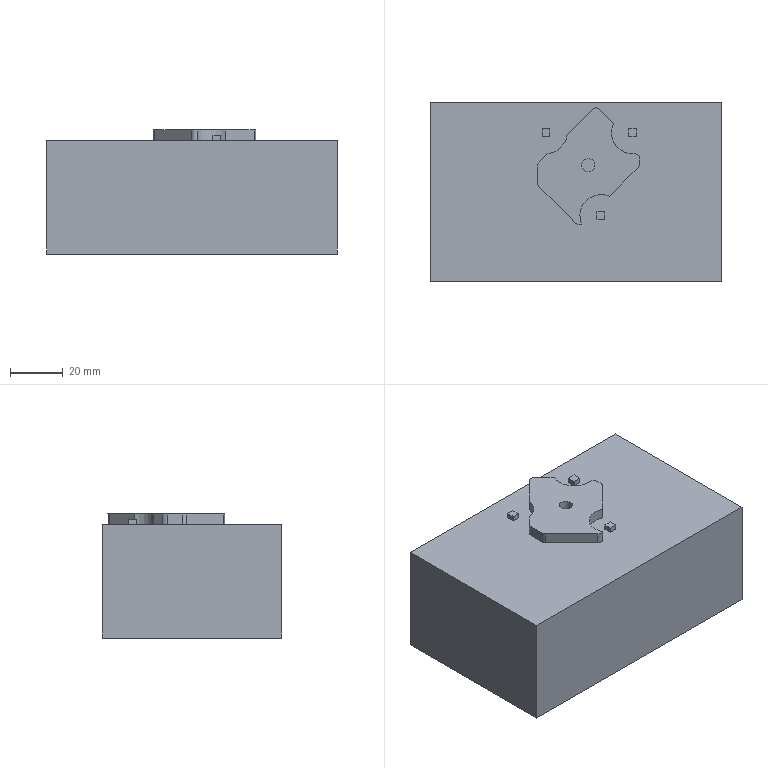Part | NX | 1 solid | 40 faces | box 110.151 x 68.163 x 47.1 mm | volume 326118 mm3 | plane 30 | cylinder 10 | commonest cylinder face diameters 4 x5 16 x3 5 x1 6 x1
STEP:
#1=CARTESIAN_POINT('',(-10.7,4.529,0.));
#2=VERTEX_POINT('',#1);
#3=CARTESIAN_POINT('',(-10.7,4.529,4.1));
#4=VERTEX_POINT('',#3);
#5=CARTESIAN_POINT('',(-10.7,4.529,0.));
#6=DIRECTION('',(0.,0.,1.));
#7=VECTOR('',#6,1000.);
#8=LINE('',#5,#7);
#9=EDGE_CURVE('',#2,#4,#8,.T.);
#10=ORIENTED_EDGE('',*,*,#9,.F.);
#11=CARTESIAN_POINT('',(-13.839,1.389,0.));
#12=VERTEX_POINT('',#11);
#13=CARTESIAN_POINT('',(7.556,22.784,0.));
#14=DIRECTION('',(0.7071,0.7071,0.));
#15=VECTOR('',#14,1000.);
#16=LINE('',#13,#15);
#17=EDGE_CURVE('',#2,#12,#16,.F.);
#18=ORIENTED_EDGE('',*,*,#17,.T.);
#19=CARTESIAN_POINT('',(-13.839,1.389,4.1));
#20=VERTEX_POINT('',#19);
#21=CARTESIAN_POINT('',(-13.839,1.389,3.));
#22=DIRECTION('',(0.,0.,-1.));
#23=VECTOR('',#22,1000.);
#24=LINE('',#21,#23);
#25=EDGE_CURVE('',#12,#20,#24,.F.);
#26=ORIENTED_EDGE('',*,*,#25,.T.);
#27=CARTESIAN_POINT('',(7.556,22.784,4.1));
#28=DIRECTION('',(0.7071,0.7071,0.));
#29=VECTOR('',#28,1000.);
#30=LINE('',#27,#29);
#31=EDGE_CURVE('',#4,#20,#30,.F.);
#32=ORIENTED_EDGE('',*,*,#31,.F.);
#33=EDGE_LOOP('',(#10,#18,#26,#32));
#34=FACE_BOUND('',#33,.T.);
#35=CARTESIAN_POINT('',(7.556,22.784,3.));
#36=DIRECTION('',(-0.7071,0.7071,0.));
#37=DIRECTION('',(-0.7071,-0.7071,0.));
#38=AXIS2_PLACEMENT_3D('',#35,#36,#37);
#39=PLANE('',#38);
#40=ADVANCED_FACE('',(#34),#39,.T.);
#41=CARTESIAN_POINT('',(23.587,-0.7827,0.));
#42=VERTEX_POINT('',#41);
#43=CARTESIAN_POINT('',(12.694,-11.676,0.));
#44=VERTEX_POINT('',#43);
#45=CARTESIAN_POINT('',(20.036,-4.333,0.));
#46=DIRECTION('',(0.7071,0.7071,0.));
#47=VECTOR('',#46,1000.);
#48=LINE('',#45,#47);
#49=EDGE_CURVE('',#42,#44,#48,.F.);
#50=ORIENTED_EDGE('',*,*,#49,.F.);
#51=CARTESIAN_POINT('',(23.587,-0.7827,4.1));
#52=VERTEX_POINT('',#51);
#53=CARTESIAN_POINT('',(23.587,-0.7827,-5.));
#54=DIRECTION('',(0.,0.,-1.));
#55=VECTOR('',#54,1000.);
#56=LINE('',#53,#55);
#57=EDGE_CURVE('',#42,#52,#56,.F.);
#58=ORIENTED_EDGE('',*,*,#57,.T.);
#59=CARTESIAN_POINT('',(12.694,-11.676,4.1));
#60=VERTEX_POINT('',#59);
#61=CARTESIAN_POINT('',(20.036,-4.333,4.1));
#62=DIRECTION('',(-0.7071,-0.7071,0.));
#63=VECTOR('',#62,1000.);
#64=LINE('',#61,#63);
#65=EDGE_CURVE('',#60,#52,#64,.F.);
#66=ORIENTED_EDGE('',*,*,#65,.F.);
#67=CARTESIAN_POINT('',(12.694,-11.676,0.));
#68=DIRECTION('',(0.,0.,1.));
#69=VECTOR('',#68,1000.);
#70=LINE('',#67,#69);
#71=EDGE_CURVE('',#44,#60,#70,.T.);
#72=ORIENTED_EDGE('',*,*,#71,.F.);
#73=EDGE_LOOP('',(#50,#58,#66,#72));
#74=FACE_BOUND('',#73,.T.);
#75=CARTESIAN_POINT('',(20.036,-4.333,-5.));
#76=DIRECTION('',(0.7071,-0.7071,0.));
#77=DIRECTION('',(0.7071,0.7071,0.));
#78=AXIS2_PLACEMENT_3D('',#75,#76,#77);
#79=PLANE('',#78);
#80=ADVANCED_FACE('',(#74),#79,.T.);
#81=CARTESIAN_POINT('',(-14.718,-0.7324,4.1));
#82=VERTEX_POINT('',#81);
#83=CARTESIAN_POINT('',(-14.718,-0.7324,0.));
#84=VERTEX_POINT('',#83);
#85=CARTESIAN_POINT('',(-14.718,-0.7324,3.));
#86=DIRECTION('',(0.,0.,-1.));
#87=VECTOR('',#86,1000.);
#88=LINE('',#85,#87);
#89=EDGE_CURVE('',#82,#84,#88,.T.);
#90=ORIENTED_EDGE('',*,*,#89,.F.);
#91=CARTESIAN_POINT('',(-11.718,-0.7324,4.1));
#92=DIRECTION('',(0.,0.,1.));
#93=DIRECTION('',(1.,0.,0.));
#94=AXIS2_PLACEMENT_3D('',#91,#92,#93);
#95=CIRCLE('',#94,3.);
#96=EDGE_CURVE('',#82,#20,#95,.F.);
#97=ORIENTED_EDGE('',*,*,#96,.T.);
#98=ORIENTED_EDGE('',*,*,#25,.F.);
#99=CARTESIAN_POINT('',(-11.718,-0.7324,0.));
#100=DIRECTION('',(0.,0.,1.));
#101=DIRECTION('',(1.,0.,0.));
#102=AXIS2_PLACEMENT_3D('',#99,#100,#101);
#103=CIRCLE('',#102,3.);
#104=EDGE_CURVE('',#84,#12,#103,.F.);
#105=ORIENTED_EDGE('',*,*,#104,.F.);
#106=EDGE_LOOP('',(#90,#97,#98,#105));
#107=FACE_BOUND('',#106,.T.);
#108=CARTESIAN_POINT('',(-11.718,-0.7324,3.));
#109=DIRECTION('',(0.,0.,-1.));
#110=DIRECTION('',(-1.,0.,0.));
#111=AXIS2_PLACEMENT_3D('',#108,#109,#110);
#112=CYLINDRICAL_SURFACE('',#111,3.);
#113=ADVANCED_FACE('',(#107),#112,.T.);
#114=CARTESIAN_POINT('',(-14.718,-6.44,0.));
#115=VERTEX_POINT('',#114);
#116=CARTESIAN_POINT('',(-14.718,0.5102,0.));
#117=DIRECTION('',(0.,1.,0.));
#118=VECTOR('',#117,1000.);
#119=LINE('',#116,#118);
#120=EDGE_CURVE('',#84,#115,#119,.F.);
#121=ORIENTED_EDGE('',*,*,#120,.T.);
#122=CARTESIAN_POINT('',(-14.718,-6.44,4.1));
#123=VERTEX_POINT('',#122);
#124=CARTESIAN_POINT('',(-14.718,-6.44,3.));
#125=DIRECTION('',(0.,0.,1.));
#126=VECTOR('',#125,1000.);
#127=LINE('',#124,#126);
#128=EDGE_CURVE('',#115,#123,#127,.T.);
#129=ORIENTED_EDGE('',*,*,#128,.T.);
#130=CARTESIAN_POINT('',(-14.718,0.5102,4.1));
#131=DIRECTION('',(0.,1.,0.));
#132=VECTOR('',#131,1000.);
#133=LINE('',#130,#132);
#134=EDGE_CURVE('',#123,#82,#133,.T.);
#135=ORIENTED_EDGE('',*,*,#134,.T.);
#136=ORIENTED_EDGE('',*,*,#89,.T.);
#137=EDGE_LOOP('',(#121,#129,#135,#136));
#138=FACE_BOUND('',#137,.T.);
#139=CARTESIAN_POINT('',(-14.718,0.5102,3.));
#140=DIRECTION('',(-1.,0.,0.));
#141=DIRECTION('',(0.,-1.,0.));
#142=AXIS2_PLACEMENT_3D('',#139,#140,#141);
#143=PLANE('',#142);
#144=ADVANCED_FACE('',(#138),#143,.T.);
#145=CARTESIAN_POINT('',(-14.132,-7.854,4.1));
#146=VERTEX_POINT('',#145);
#147=CARTESIAN_POINT('',(-0.1471,-21.839,4.1));
#148=VERTEX_POINT('',#147);
#149=CARTESIAN_POINT('',(-8.92,-13.066,4.1));
#150=DIRECTION('',(-0.7071,0.7071,0.));
#151=VECTOR('',#150,1000.);
#152=LINE('',#149,#151);
#153=EDGE_CURVE('',#146,#148,#152,.F.);
#154=ORIENTED_EDGE('',*,*,#153,.F.);
#155=CARTESIAN_POINT('',(-14.132,-7.854,0.));
#156=VERTEX_POINT('',#155);
#157=CARTESIAN_POINT('',(-14.132,-7.854,-5.));
#158=DIRECTION('',(0.,0.,1.));
#159=VECTOR('',#158,1000.);
#160=LINE('',#157,#159);
#161=EDGE_CURVE('',#146,#156,#160,.F.);
#162=ORIENTED_EDGE('',*,*,#161,.T.);
#163=CARTESIAN_POINT('',(-0.1471,-21.839,0.));
#164=VERTEX_POINT('',#163);
#165=CARTESIAN_POINT('',(-8.92,-13.066,0.));
#166=DIRECTION('',(0.7071,-0.7071,0.));
#167=VECTOR('',#166,1000.);
#168=LINE('',#165,#167);
#169=EDGE_CURVE('',#164,#156,#168,.F.);
#170=ORIENTED_EDGE('',*,*,#169,.F.);
#171=CARTESIAN_POINT('',(-0.1471,-21.839,4.1));
#172=DIRECTION('',(0.,0.,-1.));
#173=VECTOR('',#172,1000.);
#174=LINE('',#171,#173);
#175=EDGE_CURVE('',#164,#148,#174,.F.);
#176=ORIENTED_EDGE('',*,*,#175,.T.);
#177=EDGE_LOOP('',(#154,#162,#170,#176));
#178=FACE_BOUND('',#177,.T.);
#179=CARTESIAN_POINT('',(-8.92,-13.066,-5.));
#180=DIRECTION('',(-0.7071,-0.7071,0.));
#181=DIRECTION('',(0.7071,-0.7071,0.));
#182=AXIS2_PLACEMENT_3D('',#179,#180,#181);
#183=PLANE('',#182);
#184=ADVANCED_FACE('',(#178),#183,.T.);
#185=CARTESIAN_POINT('',(24.173,0.6315,0.));
#186=VERTEX_POINT('',#185);
#187=CARTESIAN_POINT('',(24.173,2.524,0.));
#188=VERTEX_POINT('',#187);
#189=CARTESIAN_POINT('',(24.173,6.167,0.));
#190=DIRECTION('',(0.,-1.,0.));
#191=VECTOR('',#190,1000.);
#192=LINE('',#189,#191);
#193=EDGE_CURVE('',#186,#188,#192,.F.);
#194=ORIENTED_EDGE('',*,*,#193,.T.);
#195=CARTESIAN_POINT('',(24.173,2.524,4.1));
#196=VERTEX_POINT('',#195);
#197=CARTESIAN_POINT('',(24.173,2.524,4.1));
#198=DIRECTION('',(0.,0.,-1.));
#199=VECTOR('',#198,1000.);
#200=LINE('',#197,#199);
#201=EDGE_CURVE('',#188,#196,#200,.F.);
#202=ORIENTED_EDGE('',*,*,#201,.T.);
#203=CARTESIAN_POINT('',(24.173,0.6315,4.1));
#204=VERTEX_POINT('',#203);
#205=CARTESIAN_POINT('',(24.173,6.167,4.1));
#206=DIRECTION('',(0.,-1.,0.));
#207=VECTOR('',#206,1000.);
#208=LINE('',#205,#207);
#209=EDGE_CURVE('',#204,#196,#208,.F.);
#210=ORIENTED_EDGE('',*,*,#209,.F.);
#211=CARTESIAN_POINT('',(24.173,0.6315,3.));
#212=DIRECTION('',(0.,0.,-1.));
#213=VECTOR('',#212,1000.);
#214=LINE('',#211,#213);
#215=EDGE_CURVE('',#204,#186,#214,.T.);
#216=ORIENTED_EDGE('',*,*,#215,.T.);
#217=EDGE_LOOP('',(#194,#202,#210,#216));
#218=FACE_BOUND('',#217,.T.);
#219=CARTESIAN_POINT('',(24.173,6.167,3.));
#220=DIRECTION('',(1.,0.,0.));
#221=DIRECTION('',(0.,1.,0.));
#222=AXIS2_PLACEMENT_3D('',#219,#220,#221);
#223=PLANE('',#222);
#224=ADVANCED_FACE('',(#218),#223,.T.);
#225=CARTESIAN_POINT('',(14.3,16.039,0.));
#226=VERTEX_POINT('',#225);
#227=CARTESIAN_POINT('',(8.97,21.37,0.));
#228=VERTEX_POINT('',#227);
#229=CARTESIAN_POINT('',(24.173,6.167,0.));
#230=DIRECTION('',(0.7071,-0.7071,0.));
#231=VECTOR('',#230,1000.);
#232=LINE('',#229,#231);
#233=EDGE_CURVE('',#226,#228,#232,.F.);
#234=ORIENTED_EDGE('',*,*,#233,.T.);
#235=CARTESIAN_POINT('',(8.97,21.37,4.1));
#236=VERTEX_POINT('',#235);
#237=CARTESIAN_POINT('',(8.97,21.37,3.));
#238=DIRECTION('',(0.,0.,-1.));
#239=VECTOR('',#238,1000.);
#240=LINE('',#237,#239);
#241=EDGE_CURVE('',#228,#236,#240,.F.);
#242=ORIENTED_EDGE('',*,*,#241,.T.);
#243=CARTESIAN_POINT('',(14.3,16.039,4.1));
#244=VERTEX_POINT('',#243);
#245=CARTESIAN_POINT('',(24.173,6.167,4.1));
#246=DIRECTION('',(0.7071,-0.7071,0.));
#247=VECTOR('',#246,1000.);
#248=LINE('',#245,#247);
#249=EDGE_CURVE('',#236,#244,#248,.T.);
#250=ORIENTED_EDGE('',*,*,#249,.T.);
#251=CARTESIAN_POINT('',(14.3,16.039,0.));
#252=DIRECTION('',(0.,0.,1.));
#253=VECTOR('',#252,1000.);
#254=LINE('',#251,#253);
#255=EDGE_CURVE('',#226,#244,#254,.T.);
#256=ORIENTED_EDGE('',*,*,#255,.F.);
#257=EDGE_LOOP('',(#234,#242,#250,#256));
#258=FACE_BOUND('',#257,.T.);
#259=CARTESIAN_POINT('',(24.173,6.167,3.));
#260=DIRECTION('',(0.7071,0.7071,0.));
#261=DIRECTION('',(-0.7071,0.7071,0.));
#262=AXIS2_PLACEMENT_3D('',#259,#260,#261);
#263=PLANE('',#262);
#264=ADVANCED_FACE('',(#258),#263,.T.);
#265=CARTESIAN_POINT('',(6.142,21.37,4.1));
#266=VERTEX_POINT('',#265);
#267=CARTESIAN_POINT('',(-3.404,11.825,4.1));
#268=VERTEX_POINT('',#267);
#269=CARTESIAN_POINT('',(7.556,22.784,4.1));
#270=DIRECTION('',(0.7071,0.7071,0.));
#271=VECTOR('',#270,1000.);
#272=LINE('',#269,#271);
#273=EDGE_CURVE('',#266,#268,#272,.F.);
#274=ORIENTED_EDGE('',*,*,#273,.F.);
#275=CARTESIAN_POINT('',(6.142,21.37,0.));
#276=VERTEX_POINT('',#275);
#277=CARTESIAN_POINT('',(6.142,21.37,3.));
#278=DIRECTION('',(0.,0.,-1.));
#279=VECTOR('',#278,1000.);
#280=LINE('',#277,#279);
#281=EDGE_CURVE('',#266,#276,#280,.T.);
#282=ORIENTED_EDGE('',*,*,#281,.T.);
#283=CARTESIAN_POINT('',(-3.404,11.825,0.));
#284=VERTEX_POINT('',#283);
#285=CARTESIAN_POINT('',(7.556,22.784,0.));
#286=DIRECTION('',(0.7071,0.7071,0.));
#287=VECTOR('',#286,1000.);
#288=LINE('',#285,#287);
#289=EDGE_CURVE('',#276,#284,#288,.F.);
#290=ORIENTED_EDGE('',*,*,#289,.T.);
#291=CARTESIAN_POINT('',(-3.404,11.825,0.));
#292=DIRECTION('',(0.,0.,1.));
#293=VECTOR('',#292,1000.);
#294=LINE('',#291,#293);
#295=EDGE_CURVE('',#268,#284,#294,.F.);
#296=ORIENTED_EDGE('',*,*,#295,.F.);
#297=EDGE_LOOP('',(#274,#282,#290,#296));
#298=FACE_BOUND('',#297,.T.);
#299=CARTESIAN_POINT('',(7.556,22.784,3.));
#300=DIRECTION('',(-0.7071,0.7071,0.));
#301=DIRECTION('',(-0.7071,-0.7071,0.));
#302=AXIS2_PLACEMENT_3D('',#299,#300,#301);
#303=PLANE('',#302);
#304=ADVANCED_FACE('',(#298),#303,.T.);
#305=ORIENTED_EDGE('',*,*,#134,.F.);
#306=CARTESIAN_POINT('',(-12.718,-6.44,4.1));
#307=DIRECTION('',(0.,0.,1.));
#308=DIRECTION('',(1.,0.,0.));
#309=AXIS2_PLACEMENT_3D('',#306,#307,#308);
#310=CIRCLE('',#309,2.);
#311=EDGE_CURVE('',#123,#146,#310,.T.);
#312=ORIENTED_EDGE('',*,*,#311,.T.);
#313=ORIENTED_EDGE('',*,*,#153,.T.);
#314=CARTESIAN_POINT('',(2.151,-22.219,4.1));
#315=VERTEX_POINT('',#314);
#316=CARTESIAN_POINT('',(1.267,-20.425,4.1));
#317=DIRECTION('',(0.,0.,1.));
#318=DIRECTION('',(1.,0.,0.));
#319=AXIS2_PLACEMENT_3D('',#316,#317,#318);
#320=CIRCLE('',#319,2.);
#321=EDGE_CURVE('',#148,#315,#320,.T.);
#322=ORIENTED_EDGE('',*,*,#321,.T.);
#323=CARTESIAN_POINT('',(9.475,-19.,4.1));
#324=DIRECTION('',(0.,0.,1.));
#325=DIRECTION('',(1.,0.,0.));
#326=AXIS2_PLACEMENT_3D('',#323,#324,#325);
#327=CIRCLE('',#326,8.);
#328=EDGE_CURVE('',#60,#315,#327,.T.);
#329=ORIENTED_EDGE('',*,*,#328,.F.);
#330=ORIENTED_EDGE('',*,*,#65,.T.);
#331=CARTESIAN_POINT('',(22.173,0.6315,4.1));
#332=DIRECTION('',(0.,0.,1.));
#333=DIRECTION('',(1.,0.,0.));
#334=AXIS2_PLACEMENT_3D('',#331,#332,#333);
#335=CIRCLE('',#334,2.);
#336=EDGE_CURVE('',#52,#204,#335,.T.);
#337=ORIENTED_EDGE('',*,*,#336,.T.);
#338=ORIENTED_EDGE('',*,*,#209,.T.);
#339=CARTESIAN_POINT('',(22.033,4.52,4.1));
#340=VERTEX_POINT('',#339);
#341=CARTESIAN_POINT('',(22.173,2.524,4.1));
#342=DIRECTION('',(0.,0.,1.));
#343=DIRECTION('',(1.,0.,0.));
#344=AXIS2_PLACEMENT_3D('',#341,#342,#343);
#345=CIRCLE('',#344,2.);
#346=EDGE_CURVE('',#196,#340,#345,.T.);
#347=ORIENTED_EDGE('',*,*,#346,.T.);
#348=CARTESIAN_POINT('',(21.475,12.5,4.1));
#349=DIRECTION('',(0.,0.,1.));
#350=DIRECTION('',(1.,0.,0.));
#351=AXIS2_PLACEMENT_3D('',#348,#349,#350);
#352=CIRCLE('',#351,8.);
#353=EDGE_CURVE('',#244,#340,#352,.T.);
#354=ORIENTED_EDGE('',*,*,#353,.F.);
#355=ORIENTED_EDGE('',*,*,#249,.F.);
#356=CARTESIAN_POINT('',(7.556,19.956,4.1));
#357=DIRECTION('',(0.,0.,1.));
#358=DIRECTION('',(1.,0.,0.));
#359=AXIS2_PLACEMENT_3D('',#356,#357,#358);
#360=CIRCLE('',#359,2.);
#361=EDGE_CURVE('',#236,#266,#360,.T.);
#362=ORIENTED_EDGE('',*,*,#361,.T.);
#363=ORIENTED_EDGE('',*,*,#273,.T.);
#364=CARTESIAN_POINT('',(-11.375,12.5,4.1));
#365=DIRECTION('',(0.,0.,1.));
#366=DIRECTION('',(1.,0.,0.));
#367=AXIS2_PLACEMENT_3D('',#364,#365,#366);
#368=CIRCLE('',#367,8.);
#369=EDGE_CURVE('',#4,#268,#368,.T.);
#370=ORIENTED_EDGE('',*,*,#369,.F.);
#371=ORIENTED_EDGE('',*,*,#31,.T.);
#372=ORIENTED_EDGE('',*,*,#96,.F.);
#373=EDGE_LOOP('',(#305,#312,#313,#322,#329,#330,#337,#338,#347,#354,#355,#362,#363,#370,#371,#372));
#374=FACE_BOUND('',#373,.T.);
#375=CARTESIAN_POINT('',(7.183,0.1472,4.1));
#376=VERTEX_POINT('',#375);
#377=CARTESIAN_POINT('',(4.683,0.1472,4.1));
#378=DIRECTION('',(0.,0.,-1.));
#379=DIRECTION('',(1.,0.,0.));
#380=AXIS2_PLACEMENT_3D('',#377,#378,#379);
#381=CIRCLE('',#380,2.5);
#382=EDGE_CURVE('',#376,#376,#381,.T.);
#383=ORIENTED_EDGE('',*,*,#382,.T.);
#384=EDGE_LOOP('',(#383));
#385=FACE_BOUND('',#384,.T.);
#386=CARTESIAN_POINT('',(4.727,-0.7272,4.1));
#387=DIRECTION('',(0.,0.,1.));
#388=DIRECTION('',(1.,0.,0.));
#389=AXIS2_PLACEMENT_3D('',#386,#387,#388);
#390=PLANE('',#389);
#391=ADVANCED_FACE('',(#374,#385),#390,.T.);
#392=ORIENTED_EDGE('',*,*,#382,.F.);
#393=EDGE_LOOP('',(#392));
#394=FACE_BOUND('',#393,.T.);
#395=CARTESIAN_POINT('',(7.183,0.1472,-15.9));
#396=VERTEX_POINT('',#395);
#397=CARTESIAN_POINT('',(4.683,0.1472,-15.9));
#398=DIRECTION('',(0.,0.,-1.));
#399=DIRECTION('',(1.,0.,0.));
#400=AXIS2_PLACEMENT_3D('',#397,#398,#399);
#401=CIRCLE('',#400,2.5);
#402=EDGE_CURVE('',#396,#396,#401,.F.);
#403=ORIENTED_EDGE('',*,*,#402,.F.);
#404=EDGE_LOOP('',(#403));
#405=FACE_BOUND('',#404,.T.);
#406=CARTESIAN_POINT('',(4.683,0.1472,-15.9));
#407=DIRECTION('',(0.,0.,1.));
#408=DIRECTION('',(1.,0.,0.));
#409=AXIS2_PLACEMENT_3D('',#406,#407,#408);
#410=CYLINDRICAL_SURFACE('',#409,2.5);
#411=ADVANCED_FACE('',(#394,#405),#410,.F.);
#412=ORIENTED_EDGE('',*,*,#353,.T.);
#413=CARTESIAN_POINT('',(22.033,4.52,0.));
#414=VERTEX_POINT('',#413);
#415=CARTESIAN_POINT('',(22.033,4.52,0.));
#416=DIRECTION('',(0.,0.,1.));
#417=VECTOR('',#416,1000.);
#418=LINE('',#415,#417);
#419=EDGE_CURVE('',#340,#414,#418,.F.);
#420=ORIENTED_EDGE('',*,*,#419,.T.);
#421=CARTESIAN_POINT('',(21.475,12.5,0.));
#422=DIRECTION('',(0.,0.,1.));
#423=DIRECTION('',(1.,0.,0.));
#424=AXIS2_PLACEMENT_3D('',#421,#422,#423);
#425=CIRCLE('',#424,8.);
#426=EDGE_CURVE('',#226,#414,#425,.T.);
#427=ORIENTED_EDGE('',*,*,#426,.F.);
#428=ORIENTED_EDGE('',*,*,#255,.T.);
#429=EDGE_LOOP('',(#412,#420,#427,#428));
#430=FACE_BOUND('',#429,.T.);
#431=CARTESIAN_POINT('',(21.475,12.5,0.));
#432=DIRECTION('',(0.,0.,1.));
#433=DIRECTION('',(1.,0.,0.));
#434=AXIS2_PLACEMENT_3D('',#431,#432,#433);
#435=CYLINDRICAL_SURFACE('',#434,8.);
#436=ADVANCED_FACE('',(#430),#435,.F.);
#437=ORIENTED_EDGE('',*,*,#71,.T.);
#438=ORIENTED_EDGE('',*,*,#328,.T.);
#439=CARTESIAN_POINT('',(2.151,-22.219,0.));
#440=VERTEX_POINT('',#439);
#441=CARTESIAN_POINT('',(2.151,-22.219,0.));
#442=DIRECTION('',(0.,0.,1.));
#443=VECTOR('',#442,1000.);
#444=LINE('',#441,#443);
#445=EDGE_CURVE('',#315,#440,#444,.F.);
#446=ORIENTED_EDGE('',*,*,#445,.T.);
#447=CARTESIAN_POINT('',(9.475,-19.,0.));
#448=DIRECTION('',(0.,0.,1.));
#449=DIRECTION('',(1.,0.,0.));
#450=AXIS2_PLACEMENT_3D('',#447,#448,#449);
#451=CIRCLE('',#450,8.);
#452=EDGE_CURVE('',#44,#440,#451,.T.);
#453=ORIENTED_EDGE('',*,*,#452,.F.);
#454=EDGE_LOOP('',(#437,#438,#446,#453));
#455=FACE_BOUND('',#454,.T.);
#456=CARTESIAN_POINT('',(9.475,-19.,0.));
#457=DIRECTION('',(0.,0.,1.));
#458=DIRECTION('',(1.,0.,0.));
#459=AXIS2_PLACEMENT_3D('',#456,#457,#458);
#460=CYLINDRICAL_SURFACE('',#459,8.);
#461=ADVANCED_FACE('',(#455),#460,.F.);
#462=ORIENTED_EDGE('',*,*,#9,.T.);
#463=ORIENTED_EDGE('',*,*,#369,.T.);
#464=ORIENTED_EDGE('',*,*,#295,.T.);
#465=CARTESIAN_POINT('',(-11.375,12.5,0.));
#466=DIRECTION('',(0.,0.,1.));
#467=DIRECTION('',(1.,0.,0.));
#468=AXIS2_PLACEMENT_3D('',#465,#466,#467);
#469=CIRCLE('',#468,8.);
#470=EDGE_CURVE('',#2,#284,#469,.T.);
#471=ORIENTED_EDGE('',*,*,#470,.F.);
#472=EDGE_LOOP('',(#462,#463,#464,#471));
#473=FACE_BOUND('',#472,.T.);
#474=CARTESIAN_POINT('',(-11.375,12.5,0.));
#475=DIRECTION('',(0.,0.,1.));
#476=DIRECTION('',(1.,0.,0.));
#477=AXIS2_PLACEMENT_3D('',#474,#475,#476);
#478=CYLINDRICAL_SURFACE('',#477,8.);
#479=ADVANCED_FACE('',(#473),#478,.F.);
#480=ORIENTED_EDGE('',*,*,#321,.F.);
#481=ORIENTED_EDGE('',*,*,#175,.F.);
#482=CARTESIAN_POINT('',(1.267,-20.425,0.));
#483=DIRECTION('',(0.,0.,1.));
#484=DIRECTION('',(1.,0.,0.));
#485=AXIS2_PLACEMENT_3D('',#482,#483,#484);
#486=CIRCLE('',#485,2.);
#487=EDGE_CURVE('',#440,#164,#486,.F.);
#488=ORIENTED_EDGE('',*,*,#487,.F.);
#489=ORIENTED_EDGE('',*,*,#445,.F.);
#490=EDGE_LOOP('',(#480,#481,#488,#489));
#491=FACE_BOUND('',#490,.T.);
#492=CARTESIAN_POINT('',(1.267,-20.425,0.));
#493=DIRECTION('',(0.,0.,1.));
#494=DIRECTION('',(1.,0.,0.));
#495=AXIS2_PLACEMENT_3D('',#492,#493,#494);
#496=CYLINDRICAL_SURFACE('',#495,2.);
#497=ADVANCED_FACE('',(#491),#496,.T.);
#498=ORIENTED_EDGE('',*,*,#336,.F.);
#499=ORIENTED_EDGE('',*,*,#57,.F.);
#500=CARTESIAN_POINT('',(22.173,0.6315,0.));
#501=DIRECTION('',(0.,0.,1.));
#502=DIRECTION('',(1.,0.,0.));
#503=AXIS2_PLACEMENT_3D('',#500,#501,#502);
#504=CIRCLE('',#503,2.);
#505=EDGE_CURVE('',#186,#42,#504,.F.);
#506=ORIENTED_EDGE('',*,*,#505,.F.);
#507=ORIENTED_EDGE('',*,*,#215,.F.);
#508=EDGE_LOOP('',(#498,#499,#506,#507));
#509=FACE_BOUND('',#508,.T.);
#510=CARTESIAN_POINT('',(22.173,0.6315,3.));
#511=DIRECTION('',(0.,0.,-1.));
#512=DIRECTION('',(-1.,0.,0.));
#513=AXIS2_PLACEMENT_3D('',#510,#511,#512);
#514=CYLINDRICAL_SURFACE('',#513,2.);
#515=ADVANCED_FACE('',(#509),#514,.T.);
#516=ORIENTED_EDGE('',*,*,#346,.F.);
#517=ORIENTED_EDGE('',*,*,#201,.F.);
#518=CARTESIAN_POINT('',(22.173,2.524,0.));
#519=DIRECTION('',(0.,0.,1.));
#520=DIRECTION('',(1.,0.,0.));
#521=AXIS2_PLACEMENT_3D('',#518,#519,#520);
#522=CIRCLE('',#521,2.);
#523=EDGE_CURVE('',#414,#188,#522,.F.);
#524=ORIENTED_EDGE('',*,*,#523,.F.);
#525=ORIENTED_EDGE('',*,*,#419,.F.);
#526=EDGE_LOOP('',(#516,#517,#524,#525));
#527=FACE_BOUND('',#526,.T.);
#528=CARTESIAN_POINT('',(22.173,2.524,0.));
#529=DIRECTION('',(0.,0.,1.));
#530=DIRECTION('',(1.,0.,0.));
#531=AXIS2_PLACEMENT_3D('',#528,#529,#530);
#532=CYLINDRICAL_SURFACE('',#531,2.);
#533=ADVANCED_FACE('',(#527),#532,.T.);
#534=ORIENTED_EDGE('',*,*,#361,.F.);
#535=ORIENTED_EDGE('',*,*,#241,.F.);
#536=CARTESIAN_POINT('',(7.556,19.956,0.));
#537=DIRECTION('',(0.,0.,1.));
#538=DIRECTION('',(1.,0.,0.));
#539=AXIS2_PLACEMENT_3D('',#536,#537,#538);
#540=CIRCLE('',#539,2.);
#541=EDGE_CURVE('',#276,#228,#540,.F.);
#542=ORIENTED_EDGE('',*,*,#541,.F.);
#543=ORIENTED_EDGE('',*,*,#281,.F.);
#544=EDGE_LOOP('',(#534,#535,#542,#543));
#545=FACE_BOUND('',#544,.T.);
#546=CARTESIAN_POINT('',(7.556,19.956,3.));
#547=DIRECTION('',(0.,0.,-1.));
#548=DIRECTION('',(-1.,0.,0.));
#549=AXIS2_PLACEMENT_3D('',#546,#547,#548);
#550=CYLINDRICAL_SURFACE('',#549,2.);
#551=ADVANCED_FACE('',(#545),#550,.T.);
#552=CARTESIAN_POINT('',(-12.718,-6.44,0.));
#553=DIRECTION('',(0.,0.,1.));
#554=DIRECTION('',(1.,0.,0.));
#555=AXIS2_PLACEMENT_3D('',#552,#553,#554);
#556=CIRCLE('',#555,2.);
#557=EDGE_CURVE('',#156,#115,#556,.F.);
#558=ORIENTED_EDGE('',*,*,#557,.F.);
#559=ORIENTED_EDGE('',*,*,#161,.F.);
#560=ORIENTED_EDGE('',*,*,#311,.F.);
#561=ORIENTED_EDGE('',*,*,#128,.F.);
#562=EDGE_LOOP('',(#558,#559,#560,#561));
#563=FACE_BOUND('',#562,.T.);
#564=CARTESIAN_POINT('',(-12.718,-6.44,3.));
#565=DIRECTION('',(0.,0.,1.));
#566=DIRECTION('',(1.,0.,0.));
#567=AXIS2_PLACEMENT_3D('',#564,#565,#566);
#568=CYLINDRICAL_SURFACE('',#567,2.);
#569=ADVANCED_FACE('',(#563),#568,.T.);
#570=CARTESIAN_POINT('',(22.975,11.,2.));
#571=VERTEX_POINT('',#570);
#572=CARTESIAN_POINT('',(22.975,11.,0.));
#573=VERTEX_POINT('',#572);
#574=CARTESIAN_POINT('',(22.975,11.,2.));
#575=DIRECTION('',(0.,0.,-1.));
#576=VECTOR('',#575,1000.);
#577=LINE('',#574,#576);
#578=EDGE_CURVE('',#571,#573,#577,.T.);
#579=ORIENTED_EDGE('',*,*,#578,.T.);
#580=CARTESIAN_POINT('',(22.975,14.,0.));
#581=VERTEX_POINT('',#580);
#582=CARTESIAN_POINT('',(22.975,14.,0.));
#583=DIRECTION('',(0.,-1.,0.));
#584=VECTOR('',#583,1000.);
#585=LINE('',#582,#584);
#586=EDGE_CURVE('',#573,#581,#585,.F.);
#587=ORIENTED_EDGE('',*,*,#586,.T.);
#588=CARTESIAN_POINT('',(22.975,14.,2.));
#589=VERTEX_POINT('',#588);
#590=CARTESIAN_POINT('',(22.975,14.,2.));
#591=DIRECTION('',(0.,0.,-1.));
#592=VECTOR('',#591,1000.);
#593=LINE('',#590,#592);
#594=EDGE_CURVE('',#589,#581,#593,.T.);
#595=ORIENTED_EDGE('',*,*,#594,.F.);
#596=CARTESIAN_POINT('',(22.975,14.,2.));
#597=DIRECTION('',(0.,-1.,0.));
#598=VECTOR('',#597,1000.);
#599=LINE('',#596,#598);
#600=EDGE_CURVE('',#589,#571,#599,.T.);
#601=ORIENTED_EDGE('',*,*,#600,.T.);
#602=EDGE_LOOP('',(#579,#587,#595,#601));
#603=FACE_BOUND('',#602,.T.);
#604=CARTESIAN_POINT('',(22.975,14.,2.));
#605=DIRECTION('',(1.,0.,0.));
#606=DIRECTION('',(0.,0.,-1.));
#607=AXIS2_PLACEMENT_3D('',#604,#605,#606);
#608=PLANE('',#607);
#609=ADVANCED_FACE('',(#603),#608,.T.);
#610=CARTESIAN_POINT('',(19.975,11.,2.));
#611=VERTEX_POINT('',#610);
#612=CARTESIAN_POINT('',(19.975,11.,0.));
#613=VERTEX_POINT('',#612);
#614=CARTESIAN_POINT('',(19.975,11.,2.));
#615=DIRECTION('',(0.,0.,-1.));
#616=VECTOR('',#615,1000.);
#617=LINE('',#614,#616);
#618=EDGE_CURVE('',#611,#613,#617,.T.);
#619=ORIENTED_EDGE('',*,*,#618,.T.);
#620=CARTESIAN_POINT('',(19.975,11.,0.));
#621=DIRECTION('',(-1.,0.,0.));
#622=VECTOR('',#621,1000.);
#623=LINE('',#620,#622);
#624=EDGE_CURVE('',#613,#573,#623,.F.);
#625=ORIENTED_EDGE('',*,*,#624,.T.);
#626=ORIENTED_EDGE('',*,*,#578,.F.);
#627=CARTESIAN_POINT('',(22.975,11.,2.));
#628=DIRECTION('',(-1.,0.,0.));
#629=VECTOR('',#628,1000.);
#630=LINE('',#627,#629);
#631=EDGE_CURVE('',#571,#611,#630,.T.);
#632=ORIENTED_EDGE('',*,*,#631,.T.);
#633=EDGE_LOOP('',(#619,#625,#626,#632));
#634=FACE_BOUND('',#633,.T.);
#635=CARTESIAN_POINT('',(22.975,11.,2.));
#636=DIRECTION('',(0.,-1.,0.));
#637=DIRECTION('',(0.,0.,-1.));
#638=AXIS2_PLACEMENT_3D('',#635,#636,#637);
#639=PLANE('',#638);
#640=ADVANCED_FACE('',(#634),#639,.T.);
#641=CARTESIAN_POINT('',(19.975,14.,2.));
#642=VERTEX_POINT('',#641);
#643=CARTESIAN_POINT('',(19.975,14.,0.));
#644=VERTEX_POINT('',#643);
#645=CARTESIAN_POINT('',(19.975,14.,2.));
#646=DIRECTION('',(0.,0.,-1.));
#647=VECTOR('',#646,1000.);
#648=LINE('',#645,#647);
#649=EDGE_CURVE('',#642,#644,#648,.T.);
#650=ORIENTED_EDGE('',*,*,#649,.T.);
#651=CARTESIAN_POINT('',(19.975,14.,0.));
#652=DIRECTION('',(0.,1.,0.));
#653=VECTOR('',#652,1000.);
#654=LINE('',#651,#653);
#655=EDGE_CURVE('',#644,#613,#654,.F.);
#656=ORIENTED_EDGE('',*,*,#655,.T.);
#657=ORIENTED_EDGE('',*,*,#618,.F.);
#658=CARTESIAN_POINT('',(19.975,11.,2.));
#659=DIRECTION('',(0.,1.,0.));
#660=VECTOR('',#659,1000.);
#661=LINE('',#658,#660);
#662=EDGE_CURVE('',#611,#642,#661,.T.);
#663=ORIENTED_EDGE('',*,*,#662,.T.);
#664=EDGE_LOOP('',(#650,#656,#657,#663));
#665=FACE_BOUND('',#664,.T.);
#666=CARTESIAN_POINT('',(19.975,11.,2.));
#667=DIRECTION('',(-1.,0.,0.));
#668=DIRECTION('',(0.,0.,1.));
#669=AXIS2_PLACEMENT_3D('',#666,#667,#668);
#670=PLANE('',#669);
#671=ADVANCED_FACE('',(#665),#670,.T.);
#672=ORIENTED_EDGE('',*,*,#594,.T.);
#673=CARTESIAN_POINT('',(19.975,14.,0.));
#674=DIRECTION('',(1.,0.,0.));
#675=VECTOR('',#674,1000.);
#676=LINE('',#673,#675);
#677=EDGE_CURVE('',#581,#644,#676,.F.);
#678=ORIENTED_EDGE('',*,*,#677,.T.);
#679=ORIENTED_EDGE('',*,*,#649,.F.);
#680=CARTESIAN_POINT('',(19.975,14.,2.));
#681=DIRECTION('',(1.,0.,0.));
#682=VECTOR('',#681,1000.);
#683=LINE('',#680,#682);
#684=EDGE_CURVE('',#642,#589,#683,.T.);
#685=ORIENTED_EDGE('',*,*,#684,.T.);
#686=EDGE_LOOP('',(#672,#678,#679,#685));
#687=FACE_BOUND('',#686,.T.);
#688=CARTESIAN_POINT('',(19.975,14.,2.));
#689=DIRECTION('',(0.,1.,0.));
#690=DIRECTION('',(0.,0.,1.));
#691=AXIS2_PLACEMENT_3D('',#688,#689,#690);
#692=PLANE('',#691);
#693=ADVANCED_FACE('',(#687),#692,.T.);
#694=ORIENTED_EDGE('',*,*,#631,.F.);
#695=ORIENTED_EDGE('',*,*,#600,.F.);
#696=ORIENTED_EDGE('',*,*,#684,.F.);
#697=ORIENTED_EDGE('',*,*,#662,.F.);
#698=EDGE_LOOP('',(#694,#695,#696,#697));
#699=FACE_BOUND('',#698,.T.);
#700=CARTESIAN_POINT('',(0.,0.,2.));
#701=DIRECTION('',(0.,0.,-1.));
#702=DIRECTION('',(-1.,0.,0.));
#703=AXIS2_PLACEMENT_3D('',#700,#701,#702);
#704=PLANE('',#703);
#705=ADVANCED_FACE('',(#699),#704,.F.);
#706=CARTESIAN_POINT('',(10.975,-17.5,2.));
#707=VERTEX_POINT('',#706);
#708=CARTESIAN_POINT('',(10.975,-17.5,0.));
#709=VERTEX_POINT('',#708);
#710=CARTESIAN_POINT('',(10.975,-17.5,2.));
#711=DIRECTION('',(0.,0.,-1.));
#712=VECTOR('',#711,1000.);
#713=LINE('',#710,#712);
#714=EDGE_CURVE('',#707,#709,#713,.T.);
#715=ORIENTED_EDGE('',*,*,#714,.T.);
#716=CARTESIAN_POINT('',(7.975,-17.5,0.));
#717=VERTEX_POINT('',#716);
#718=CARTESIAN_POINT('',(7.975,-17.5,0.));
#719=DIRECTION('',(1.,0.,0.));
#720=VECTOR('',#719,1000.);
#721=LINE('',#718,#720);
#722=EDGE_CURVE('',#709,#717,#721,.F.);
#723=ORIENTED_EDGE('',*,*,#722,.T.);
#724=CARTESIAN_POINT('',(7.975,-17.5,2.));
#725=VERTEX_POINT('',#724);
#726=CARTESIAN_POINT('',(7.975,-17.5,2.));
#727=DIRECTION('',(0.,0.,-1.));
#728=VECTOR('',#727,1000.);
#729=LINE('',#726,#728);
#730=EDGE_CURVE('',#725,#717,#729,.T.);
#731=ORIENTED_EDGE('',*,*,#730,.F.);
#732=CARTESIAN_POINT('',(7.975,-17.5,2.));
#733=DIRECTION('',(1.,0.,0.));
#734=VECTOR('',#733,1000.);
#735=LINE('',#732,#734);
#736=EDGE_CURVE('',#725,#707,#735,.T.);
#737=ORIENTED_EDGE('',*,*,#736,.T.);
#738=EDGE_LOOP('',(#715,#723,#731,#737));
#739=FACE_BOUND('',#738,.T.);
#740=CARTESIAN_POINT('',(7.975,-17.5,2.));
#741=DIRECTION('',(0.,1.,0.));
#742=DIRECTION('',(0.,0.,1.));
#743=AXIS2_PLACEMENT_3D('',#740,#741,#742);
#744=PLANE('',#743);
#745=ADVANCED_FACE('',(#739),#744,.T.);
#746=CARTESIAN_POINT('',(10.975,-20.5,2.));
#747=VERTEX_POINT('',#746);
#748=CARTESIAN_POINT('',(10.975,-20.5,0.));
#749=VERTEX_POINT('',#748);
#750=CARTESIAN_POINT('',(10.975,-20.5,2.));
#751=DIRECTION('',(0.,0.,-1.));
#752=VECTOR('',#751,1000.);
#753=LINE('',#750,#752);
#754=EDGE_CURVE('',#747,#749,#753,.T.);
#755=ORIENTED_EDGE('',*,*,#754,.T.);
#756=CARTESIAN_POINT('',(10.975,-17.5,0.));
#757=DIRECTION('',(0.,-1.,0.));
#758=VECTOR('',#757,1000.);
#759=LINE('',#756,#758);
#760=EDGE_CURVE('',#749,#709,#759,.F.);
#761=ORIENTED_EDGE('',*,*,#760,.T.);
#762=ORIENTED_EDGE('',*,*,#714,.F.);
#763=CARTESIAN_POINT('',(10.975,-17.5,2.));
#764=DIRECTION('',(0.,-1.,0.));
#765=VECTOR('',#764,1000.);
#766=LINE('',#763,#765);
#767=EDGE_CURVE('',#707,#747,#766,.T.);
#768=ORIENTED_EDGE('',*,*,#767,.T.);
#769=EDGE_LOOP('',(#755,#761,#762,#768));
#770=FACE_BOUND('',#769,.T.);
#771=CARTESIAN_POINT('',(10.975,-17.5,2.));
#772=DIRECTION('',(1.,0.,0.));
#773=DIRECTION('',(0.,0.,-1.));
#774=AXIS2_PLACEMENT_3D('',#771,#772,#773);
#775=PLANE('',#774);
#776=ADVANCED_FACE('',(#770),#775,.T.);
#777=CARTESIAN_POINT('',(7.975,-20.5,2.));
#778=VERTEX_POINT('',#777);
#779=CARTESIAN_POINT('',(7.975,-20.5,0.));
#780=VERTEX_POINT('',#779);
#781=CARTESIAN_POINT('',(7.975,-20.5,2.));
#782=DIRECTION('',(0.,0.,-1.));
#783=VECTOR('',#782,1000.);
#784=LINE('',#781,#783);
#785=EDGE_CURVE('',#778,#780,#784,.T.);
#786=ORIENTED_EDGE('',*,*,#785,.T.);
#787=CARTESIAN_POINT('',(7.975,-20.5,0.));
#788=DIRECTION('',(-1.,0.,0.));
#789=VECTOR('',#788,1000.);
#790=LINE('',#787,#789);
#791=EDGE_CURVE('',#780,#749,#790,.F.);
#792=ORIENTED_EDGE('',*,*,#791,.T.);
#793=ORIENTED_EDGE('',*,*,#754,.F.);
#794=CARTESIAN_POINT('',(10.975,-20.5,2.));
#795=DIRECTION('',(-1.,0.,0.));
#796=VECTOR('',#795,1000.);
#797=LINE('',#794,#796);
#798=EDGE_CURVE('',#747,#778,#797,.T.);
#799=ORIENTED_EDGE('',*,*,#798,.T.);
#800=EDGE_LOOP('',(#786,#792,#793,#799));
#801=FACE_BOUND('',#800,.T.);
#802=CARTESIAN_POINT('',(10.975,-20.5,2.));
#803=DIRECTION('',(0.,-1.,0.));
#804=DIRECTION('',(0.,0.,-1.));
#805=AXIS2_PLACEMENT_3D('',#802,#803,#804);
#806=PLANE('',#805);
#807=ADVANCED_FACE('',(#801),#806,.T.);
#808=ORIENTED_EDGE('',*,*,#730,.T.);
#809=CARTESIAN_POINT('',(7.975,-17.5,0.));
#810=DIRECTION('',(0.,1.,0.));
#811=VECTOR('',#810,1000.);
#812=LINE('',#809,#811);
#813=EDGE_CURVE('',#717,#780,#812,.F.);
#814=ORIENTED_EDGE('',*,*,#813,.T.);
#815=ORIENTED_EDGE('',*,*,#785,.F.);
#816=CARTESIAN_POINT('',(7.975,-20.5,2.));
#817=DIRECTION('',(0.,1.,0.));
#818=VECTOR('',#817,1000.);
#819=LINE('',#816,#818);
#820=EDGE_CURVE('',#778,#725,#819,.T.);
#821=ORIENTED_EDGE('',*,*,#820,.T.);
#822=EDGE_LOOP('',(#808,#814,#815,#821));
#823=FACE_BOUND('',#822,.T.);
#824=CARTESIAN_POINT('',(7.975,-20.5,2.));
#825=DIRECTION('',(-1.,0.,0.));
#826=DIRECTION('',(0.,0.,1.));
#827=AXIS2_PLACEMENT_3D('',#824,#825,#826);
#828=PLANE('',#827);
#829=ADVANCED_FACE('',(#823),#828,.T.);
#830=ORIENTED_EDGE('',*,*,#767,.F.);
#831=ORIENTED_EDGE('',*,*,#736,.F.);
#832=ORIENTED_EDGE('',*,*,#820,.F.);
#833=ORIENTED_EDGE('',*,*,#798,.F.);
#834=EDGE_LOOP('',(#830,#831,#832,#833));
#835=FACE_BOUND('',#834,.T.);
#836=CARTESIAN_POINT('',(0.,0.,2.));
#837=DIRECTION('',(0.,0.,-1.));
#838=DIRECTION('',(-1.,0.,0.));
#839=AXIS2_PLACEMENT_3D('',#836,#837,#838);
#840=PLANE('',#839);
#841=ADVANCED_FACE('',(#835),#840,.F.);
#842=CARTESIAN_POINT('',(-55.075,24.081,-43.));
#843=VERTEX_POINT('',#842);
#844=CARTESIAN_POINT('',(-55.075,24.081,0.));
#845=VERTEX_POINT('',#844);
#846=CARTESIAN_POINT('',(-55.075,24.081,-38.));
#847=DIRECTION('',(0.,0.,1.));
#848=VECTOR('',#847,1000.);
#849=LINE('',#846,#848);
#850=EDGE_CURVE('',#843,#845,#849,.T.);
#851=ORIENTED_EDGE('',*,*,#850,.T.);
#852=CARTESIAN_POINT('',(55.075,24.081,0.));
#853=VERTEX_POINT('',#852);
#854=CARTESIAN_POINT('',(0.,24.081,0.));
#855=DIRECTION('',(1.,0.,0.));
#856=VECTOR('',#855,1000.);
#857=LINE('',#854,#856);
#858=EDGE_CURVE('',#853,#845,#857,.F.);
#859=ORIENTED_EDGE('',*,*,#858,.F.);
#860=CARTESIAN_POINT('',(55.075,24.081,-43.));
#861=VERTEX_POINT('',#860);
#862=CARTESIAN_POINT('',(55.075,24.081,-38.));
#863=DIRECTION('',(0.,0.,1.));
#864=VECTOR('',#863,1000.);
#865=LINE('',#862,#864);
#866=EDGE_CURVE('',#861,#853,#865,.T.);
#867=ORIENTED_EDGE('',*,*,#866,.F.);
#868=CARTESIAN_POINT('',(0.,24.081,-43.));
#869=DIRECTION('',(-1.,0.,0.));
#870=VECTOR('',#869,1000.);
#871=LINE('',#868,#870);
#872=EDGE_CURVE('',#861,#843,#871,.T.);
#873=ORIENTED_EDGE('',*,*,#872,.T.);
#874=EDGE_LOOP('',(#851,#859,#867,#873));
#875=FACE_BOUND('',#874,.T.);
#876=CARTESIAN_POINT('',(0.,24.081,-38.));
#877=DIRECTION('',(0.,1.,0.));
#878=DIRECTION('',(0.,0.,1.));
#879=AXIS2_PLACEMENT_3D('',#876,#877,#878);
#880=PLANE('',#879);
#881=ADVANCED_FACE('',(#875),#880,.T.);
#882=CARTESIAN_POINT('',(55.075,-44.081,-43.));
#883=VERTEX_POINT('',#882);
#884=CARTESIAN_POINT('',(55.075,-44.081,0.));
#885=VERTEX_POINT('',#884);
#886=CARTESIAN_POINT('',(55.075,-44.081,-38.));
#887=DIRECTION('',(0.,0.,1.));
#888=VECTOR('',#887,1000.);
#889=LINE('',#886,#888);
#890=EDGE_CURVE('',#883,#885,#889,.T.);
#891=ORIENTED_EDGE('',*,*,#890,.T.);
#892=CARTESIAN_POINT('',(-55.075,-44.081,0.));
#893=VERTEX_POINT('',#892);
#894=CARTESIAN_POINT('',(0.,-44.081,0.));
#895=DIRECTION('',(-1.,0.,0.));
#896=VECTOR('',#895,1000.);
#897=LINE('',#894,#896);
#898=EDGE_CURVE('',#885,#893,#897,.T.);
#899=ORIENTED_EDGE('',*,*,#898,.T.);
#900=CARTESIAN_POINT('',(-55.075,-44.081,-43.));
#901=VERTEX_POINT('',#900);
#902=CARTESIAN_POINT('',(-55.075,-44.081,-38.));
#903=DIRECTION('',(0.,0.,1.));
#904=VECTOR('',#903,1000.);
#905=LINE('',#902,#904);
#906=EDGE_CURVE('',#901,#893,#905,.T.);
#907=ORIENTED_EDGE('',*,*,#906,.F.);
#908=CARTESIAN_POINT('',(0.,-44.081,-43.));
#909=DIRECTION('',(1.,0.,0.));
#910=VECTOR('',#909,1000.);
#911=LINE('',#908,#910);
#912=EDGE_CURVE('',#901,#883,#911,.T.);
#913=ORIENTED_EDGE('',*,*,#912,.T.);
#914=EDGE_LOOP('',(#891,#899,#907,#913));
#915=FACE_BOUND('',#914,.T.);
#916=CARTESIAN_POINT('',(0.,-44.081,-38.));
#917=DIRECTION('',(0.,-1.,0.));
#918=DIRECTION('',(0.,0.,-1.));
#919=AXIS2_PLACEMENT_3D('',#916,#917,#918);
#920=PLANE('',#919);
#921=ADVANCED_FACE('',(#915),#920,.T.);
#922=ORIENTED_EDGE('',*,*,#866,.T.);
#923=CARTESIAN_POINT('',(55.075,0.,0.));
#924=DIRECTION('',(0.,-1.,0.));
#925=VECTOR('',#924,1000.);
#926=LINE('',#923,#925);
#927=EDGE_CURVE('',#853,#885,#926,.T.);
#928=ORIENTED_EDGE('',*,*,#927,.T.);
#929=ORIENTED_EDGE('',*,*,#890,.F.);
#930=CARTESIAN_POINT('',(55.075,0.,-43.));
#931=DIRECTION('',(0.,1.,0.));
#932=VECTOR('',#931,1000.);
#933=LINE('',#930,#932);
#934=EDGE_CURVE('',#883,#861,#933,.T.);
#935=ORIENTED_EDGE('',*,*,#934,.T.);
#936=EDGE_LOOP('',(#922,#928,#929,#935));
#937=FACE_BOUND('',#936,.T.);
#938=CARTESIAN_POINT('',(55.075,0.,-38.));
#939=DIRECTION('',(1.,0.,0.));
#940=DIRECTION('',(0.,0.,-1.));
#941=AXIS2_PLACEMENT_3D('',#938,#939,#940);
#942=PLANE('',#941);
#943=ADVANCED_FACE('',(#937),#942,.T.);
#944=ORIENTED_EDGE('',*,*,#906,.T.);
#945=CARTESIAN_POINT('',(-55.075,0.,0.));
#946=DIRECTION('',(0.,1.,0.));
#947=VECTOR('',#946,1000.);
#948=LINE('',#945,#947);
#949=EDGE_CURVE('',#893,#845,#948,.T.);
#950=ORIENTED_EDGE('',*,*,#949,.T.);
#951=ORIENTED_EDGE('',*,*,#850,.F.);
#952=CARTESIAN_POINT('',(-55.075,0.,-43.));
#953=DIRECTION('',(0.,-1.,0.));
#954=VECTOR('',#953,1000.);
#955=LINE('',#952,#954);
#956=EDGE_CURVE('',#843,#901,#955,.T.);
#957=ORIENTED_EDGE('',*,*,#956,.T.);
#958=EDGE_LOOP('',(#944,#950,#951,#957));
#959=FACE_BOUND('',#958,.T.);
#960=CARTESIAN_POINT('',(-55.075,0.,-38.));
#961=DIRECTION('',(-1.,0.,0.));
#962=DIRECTION('',(0.,0.,1.));
#963=AXIS2_PLACEMENT_3D('',#960,#961,#962);
#964=PLANE('',#963);
#965=ADVANCED_FACE('',(#959),#964,.T.);
#966=ORIENTED_EDGE('',*,*,#934,.F.);
#967=ORIENTED_EDGE('',*,*,#912,.F.);
#968=ORIENTED_EDGE('',*,*,#956,.F.);
#969=ORIENTED_EDGE('',*,*,#872,.F.);
#970=EDGE_LOOP('',(#966,#967,#968,#969));
#971=FACE_BOUND('',#970,.T.);
#972=CARTESIAN_POINT('',(0.,0.,-43.));
#973=DIRECTION('',(0.,0.,-1.));
#974=DIRECTION('',(-1.,0.,0.));
#975=AXIS2_PLACEMENT_3D('',#972,#973,#974);
#976=PLANE('',#975);
#977=ADVANCED_FACE('',(#971),#976,.T.);
#978=ORIENTED_EDGE('',*,*,#487,.T.);
#979=ORIENTED_EDGE('',*,*,#169,.T.);
#980=ORIENTED_EDGE('',*,*,#557,.T.);
#981=ORIENTED_EDGE('',*,*,#120,.F.);
#982=ORIENTED_EDGE('',*,*,#104,.T.);
#983=ORIENTED_EDGE('',*,*,#17,.F.);
#984=ORIENTED_EDGE('',*,*,#470,.T.);
#985=ORIENTED_EDGE('',*,*,#289,.F.);
#986=ORIENTED_EDGE('',*,*,#541,.T.);
#987=ORIENTED_EDGE('',*,*,#233,.F.);
#988=ORIENTED_EDGE('',*,*,#426,.T.);
#989=ORIENTED_EDGE('',*,*,#523,.T.);
#990=ORIENTED_EDGE('',*,*,#193,.F.);
#991=ORIENTED_EDGE('',*,*,#505,.T.);
#992=ORIENTED_EDGE('',*,*,#49,.T.);
#993=ORIENTED_EDGE('',*,*,#452,.T.);
#994=EDGE_LOOP('',(#978,#979,#980,#981,#982,#983,#984,#985,#986,#987,#988,#989,#990,#991,#992,#993));
#995=FACE_BOUND('',#994,.T.);
#996=CARTESIAN_POINT('',(-12.725,11.,0.));
#997=VERTEX_POINT('',#996);
#998=CARTESIAN_POINT('',(-10.025,11.,0.));
#999=VERTEX_POINT('',#998);
#1000=CARTESIAN_POINT('',(-13.025,11.,0.));
#1001=DIRECTION('',(-1.,0.,0.));
#1002=VECTOR('',#1001,1000.);
#1003=LINE('',#1000,#1002);
#1004=EDGE_CURVE('',#997,#999,#1003,.F.);
#1005=ORIENTED_EDGE('',*,*,#1004,.F.);
#1006=CARTESIAN_POINT('',(-12.725,14.,0.));
#1007=VERTEX_POINT('',#1006);
#1008=CARTESIAN_POINT('',(-12.725,14.,0.));
#1009=DIRECTION('',(0.,-1.,0.));
#1010=VECTOR('',#1009,1000.);
#1011=LINE('',#1008,#1010);
#1012=EDGE_CURVE('',#997,#1007,#1011,.F.);
#1013=ORIENTED_EDGE('',*,*,#1012,.T.);
#1014=CARTESIAN_POINT('',(-10.025,14.,0.));
#1015=VERTEX_POINT('',#1014);
#1016=CARTESIAN_POINT('',(-13.025,14.,0.));
#1017=DIRECTION('',(1.,0.,0.));
#1018=VECTOR('',#1017,1000.);
#1019=LINE('',#1016,#1018);
#1020=EDGE_CURVE('',#1015,#1007,#1019,.F.);
#1021=ORIENTED_EDGE('',*,*,#1020,.F.);
#1022=CARTESIAN_POINT('',(-10.025,14.,0.));
#1023=DIRECTION('',(0.,-1.,0.));
#1024=VECTOR('',#1023,1000.);
#1025=LINE('',#1022,#1024);
#1026=EDGE_CURVE('',#999,#1015,#1025,.F.);
#1027=ORIENTED_EDGE('',*,*,#1026,.F.);
#1028=EDGE_LOOP('',(#1005,#1013,#1021,#1027));
#1029=FACE_BOUND('',#1028,.T.);
#1030=ORIENTED_EDGE('',*,*,#624,.F.);
#1031=ORIENTED_EDGE('',*,*,#655,.F.);
#1032=ORIENTED_EDGE('',*,*,#677,.F.);
#1033=ORIENTED_EDGE('',*,*,#586,.F.);
#1034=EDGE_LOOP('',(#1030,#1031,#1032,#1033));
#1035=FACE_BOUND('',#1034,.T.);
#1036=ORIENTED_EDGE('',*,*,#760,.F.);
#1037=ORIENTED_EDGE('',*,*,#791,.F.);
#1038=ORIENTED_EDGE('',*,*,#813,.F.);
#1039=ORIENTED_EDGE('',*,*,#722,.F.);
#1040=EDGE_LOOP('',(#1036,#1037,#1038,#1039));
#1041=FACE_BOUND('',#1040,.T.);
#1042=ORIENTED_EDGE('',*,*,#927,.F.);
#1043=ORIENTED_EDGE('',*,*,#858,.T.);
#1044=ORIENTED_EDGE('',*,*,#949,.F.);
#1045=ORIENTED_EDGE('',*,*,#898,.F.);
#1046=EDGE_LOOP('',(#1042,#1043,#1044,#1045));
#1047=FACE_BOUND('',#1046,.T.);
#1048=CARTESIAN_POINT('',(-29.025,20.886,0.));
#1049=DIRECTION('',(0.,0.,-1.));
#1050=DIRECTION('',(-1.,0.,0.));
#1051=AXIS2_PLACEMENT_3D('',#1048,#1049,#1050);
#1052=PLANE('',#1051);
#1053=ADVANCED_FACE('',(#995,#1029,#1035,#1041,#1047),#1052,.F.);
#1054=CARTESIAN_POINT('',(-12.725,11.,2.));
#1055=VERTEX_POINT('',#1054);
#1056=CARTESIAN_POINT('',(-12.725,11.,2.));
#1057=DIRECTION('',(0.,0.,-1.));
#1058=VECTOR('',#1057,1000.);
#1059=LINE('',#1056,#1058);
#1060=EDGE_CURVE('',#1055,#997,#1059,.T.);
#1061=ORIENTED_EDGE('',*,*,#1060,.T.);
#1062=ORIENTED_EDGE('',*,*,#1004,.T.);
#1063=CARTESIAN_POINT('',(-10.025,11.,2.));
#1064=VERTEX_POINT('',#1063);
#1065=CARTESIAN_POINT('',(-10.025,11.,2.));
#1066=DIRECTION('',(0.,0.,-1.));
#1067=VECTOR('',#1066,1000.);
#1068=LINE('',#1065,#1067);
#1069=EDGE_CURVE('',#1064,#999,#1068,.T.);
#1070=ORIENTED_EDGE('',*,*,#1069,.F.);
#1071=CARTESIAN_POINT('',(-13.025,11.,2.));
#1072=DIRECTION('',(1.,0.,0.));
#1073=VECTOR('',#1072,1000.);
#1074=LINE('',#1071,#1073);
#1075=EDGE_CURVE('',#1055,#1064,#1074,.T.);
#1076=ORIENTED_EDGE('',*,*,#1075,.F.);
#1077=EDGE_LOOP('',(#1061,#1062,#1070,#1076));
#1078=FACE_BOUND('',#1077,.T.);
#1079=CARTESIAN_POINT('',(-13.025,11.,2.));
#1080=DIRECTION('',(0.,1.,0.));
#1081=DIRECTION('',(0.,0.,1.));
#1082=AXIS2_PLACEMENT_3D('',#1079,#1080,#1081);
#1083=PLANE('',#1082);
#1084=ADVANCED_FACE('',(#1078),#1083,.F.);
#1085=ORIENTED_EDGE('',*,*,#1012,.F.);
#1086=ORIENTED_EDGE('',*,*,#1060,.F.);
#1087=CARTESIAN_POINT('',(-12.725,14.,2.));
#1088=VERTEX_POINT('',#1087);
#1089=CARTESIAN_POINT('',(-12.725,14.,2.));
#1090=DIRECTION('',(0.,-1.,0.));
#1091=VECTOR('',#1090,1000.);
#1092=LINE('',#1089,#1091);
#1093=EDGE_CURVE('',#1088,#1055,#1092,.T.);
#1094=ORIENTED_EDGE('',*,*,#1093,.F.);
#1095=CARTESIAN_POINT('',(-12.725,14.,2.));
#1096=DIRECTION('',(0.,0.,-1.));
#1097=VECTOR('',#1096,1000.);
#1098=LINE('',#1095,#1097);
#1099=EDGE_CURVE('',#1088,#1007,#1098,.T.);
#1100=ORIENTED_EDGE('',*,*,#1099,.T.);
#1101=EDGE_LOOP('',(#1085,#1086,#1094,#1100));
#1102=FACE_BOUND('',#1101,.T.);
#1103=CARTESIAN_POINT('',(-12.725,14.,-2.25));
#1104=DIRECTION('',(-1.,0.,0.));
#1105=DIRECTION('',(0.,-1.,0.));
#1106=AXIS2_PLACEMENT_3D('',#1103,#1104,#1105);
#1107=PLANE('',#1106);
#1108=ADVANCED_FACE('',(#1102),#1107,.T.);
#1109=CARTESIAN_POINT('',(-10.025,14.,2.));
#1110=VERTEX_POINT('',#1109);
#1111=CARTESIAN_POINT('',(-10.025,14.,2.));
#1112=DIRECTION('',(0.,0.,-1.));
#1113=VECTOR('',#1112,1000.);
#1114=LINE('',#1111,#1113);
#1115=EDGE_CURVE('',#1110,#1015,#1114,.T.);
#1116=ORIENTED_EDGE('',*,*,#1115,.T.);
#1117=ORIENTED_EDGE('',*,*,#1020,.T.);
#1118=ORIENTED_EDGE('',*,*,#1099,.F.);
#1119=CARTESIAN_POINT('',(-10.025,14.,2.));
#1120=DIRECTION('',(-1.,0.,0.));
#1121=VECTOR('',#1120,1000.);
#1122=LINE('',#1119,#1121);
#1123=EDGE_CURVE('',#1110,#1088,#1122,.T.);
#1124=ORIENTED_EDGE('',*,*,#1123,.F.);
#1125=EDGE_LOOP('',(#1116,#1117,#1118,#1124));
#1126=FACE_BOUND('',#1125,.T.);
#1127=CARTESIAN_POINT('',(-10.025,14.,2.));
#1128=DIRECTION('',(0.,-1.,0.));
#1129=DIRECTION('',(0.,0.,-1.));
#1130=AXIS2_PLACEMENT_3D('',#1127,#1128,#1129);
#1131=PLANE('',#1130);
#1132=ADVANCED_FACE('',(#1126),#1131,.F.);
#1133=ORIENTED_EDGE('',*,*,#1069,.T.);
#1134=ORIENTED_EDGE('',*,*,#1026,.T.);
#1135=ORIENTED_EDGE('',*,*,#1115,.F.);
#1136=CARTESIAN_POINT('',(-10.025,11.,2.));
#1137=DIRECTION('',(0.,1.,0.));
#1138=VECTOR('',#1137,1000.);
#1139=LINE('',#1136,#1138);
#1140=EDGE_CURVE('',#1064,#1110,#1139,.T.);
#1141=ORIENTED_EDGE('',*,*,#1140,.F.);
#1142=EDGE_LOOP('',(#1133,#1134,#1135,#1141));
#1143=FACE_BOUND('',#1142,.T.);
#1144=CARTESIAN_POINT('',(-10.025,11.,2.));
#1145=DIRECTION('',(-1.,0.,0.));
#1146=DIRECTION('',(0.,0.,1.));
#1147=AXIS2_PLACEMENT_3D('',#1144,#1145,#1146);
#1148=PLANE('',#1147);
#1149=ADVANCED_FACE('',(#1143),#1148,.F.);
#1150=ORIENTED_EDGE('',*,*,#1093,.T.);
#1151=ORIENTED_EDGE('',*,*,#1075,.T.);
#1152=ORIENTED_EDGE('',*,*,#1140,.T.);
#1153=ORIENTED_EDGE('',*,*,#1123,.T.);
#1154=EDGE_LOOP('',(#1150,#1151,#1152,#1153));
#1155=FACE_BOUND('',#1154,.T.);
#1156=CARTESIAN_POINT('',(0.,0.,2.));
#1157=DIRECTION('',(0.,0.,1.));
#1158=DIRECTION('',(1.,0.,0.));
#1159=AXIS2_PLACEMENT_3D('',#1156,#1157,#1158);
#1160=PLANE('',#1159);
#1161=ADVANCED_FACE('',(#1155),#1160,.T.);
#1162=ORIENTED_EDGE('',*,*,#402,.T.);
#1163=EDGE_LOOP('',(#1162));
#1164=FACE_BOUND('',#1163,.T.);
#1165=CARTESIAN_POINT('',(4.683,0.1472,-15.9));
#1166=DIRECTION('',(0.,0.,-1.));
#1167=DIRECTION('',(-1.,0.,0.));
#1168=AXIS2_PLACEMENT_3D('',#1165,#1166,#1167);
#1169=PLANE('',#1168);
#1170=ADVANCED_FACE('',(#1164),#1169,.F.);
#1171=CLOSED_SHELL('',(#40,#80,#113,#144,#184,#224,#264,#304,#391,#411,#436,#461,#479,#497,#515,#533,#551,#569,#609,#640,#671,#693,#705,#745,#776,#807,#829,#841,#881,#921,#943,#965,#977,#1053,#1084,#1108,#1132,#1149,#1161,#1170));
#1172=MANIFOLD_SOLID_BREP('',#1171);
#1173=(LENGTH_UNIT()NAMED_UNIT(*)SI_UNIT(.MILLI.,.METRE.));
#1174=UNCERTAINTY_MEASURE_WITH_UNIT(LENGTH_MEASURE(0.00001),#1173,'','');
#1175=(NAMED_UNIT(*)PLANE_ANGLE_UNIT()SI_UNIT($,.RADIAN.));
#1176=(NAMED_UNIT(*)SI_UNIT($,.STERADIAN.)SOLID_ANGLE_UNIT());
#1177=(GEOMETRIC_REPRESENTATION_CONTEXT(3)GLOBAL_UNCERTAINTY_ASSIGNED_CONTEXT((#1174))GLOBAL_UNIT_ASSIGNED_CONTEXT((#1173,#1175,#1176))REPRESENTATION_CONTEXT('',''));
#1178=ADVANCED_BREP_SHAPE_REPRESENTATION('',(#1172),#1177);